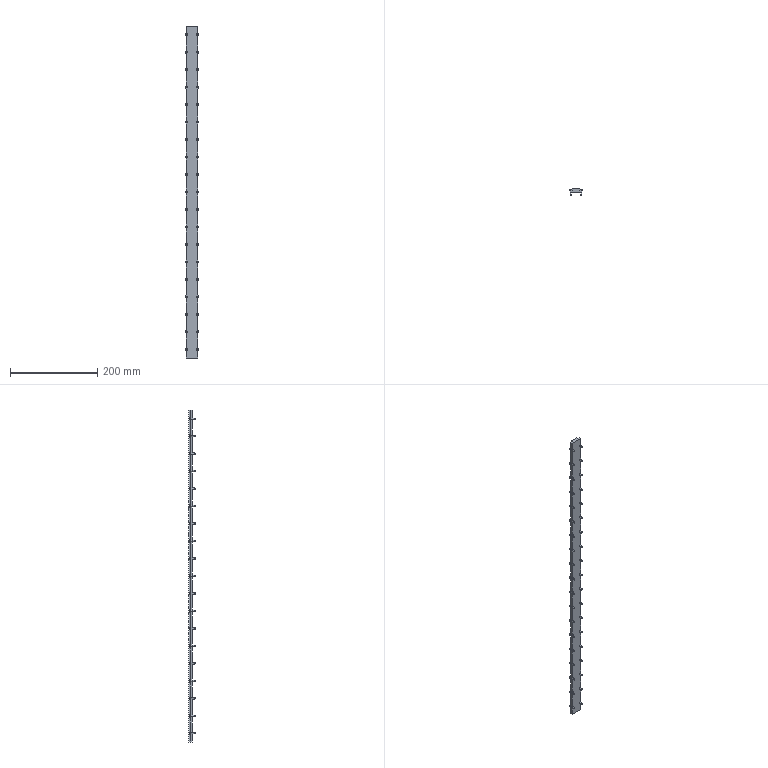Part | STEP file | BODY2_E-RAM6-S-640-ME30-C5 | 1 solid | 694 faces | box 29.5 x 14 x 759.7 mm | volume 139980 mm3 | plane 504 | cylinder 114 | torus 38 | cone 38 | commonest cylinder face diameters 3 x38 4 x38 5.5 x38